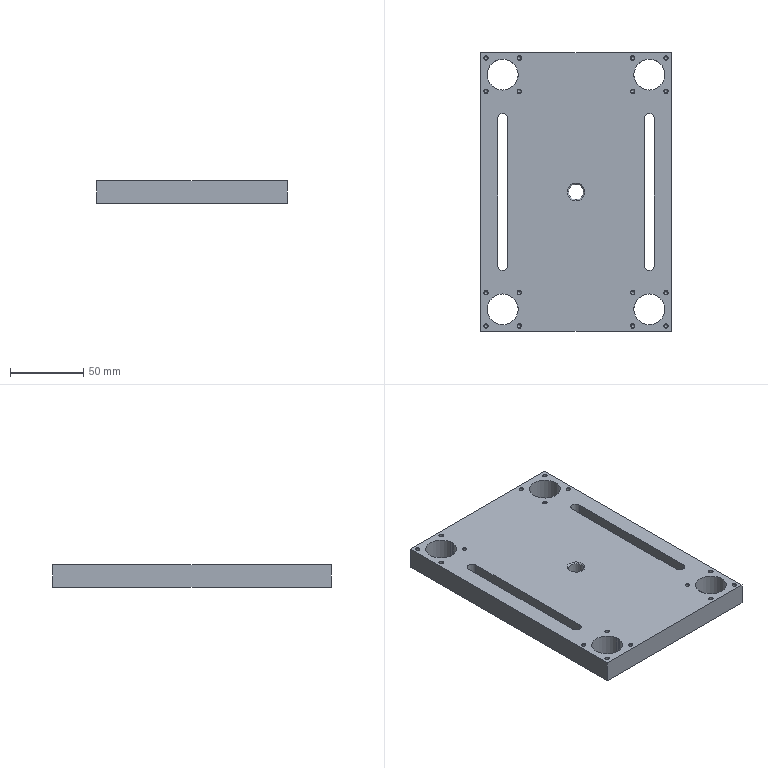Part | STEP file | YBQDJ-YY-7 | 1 solid | 81 faces | box 130 x 190 x 15 mm | volume 325427 mm3 | cylinder 37 | cone 34 | plane 10 | commonest cylinder face diameters 2.5 x16 4 x8 1 x4 7 x4 21.01 x4 10.3 x1